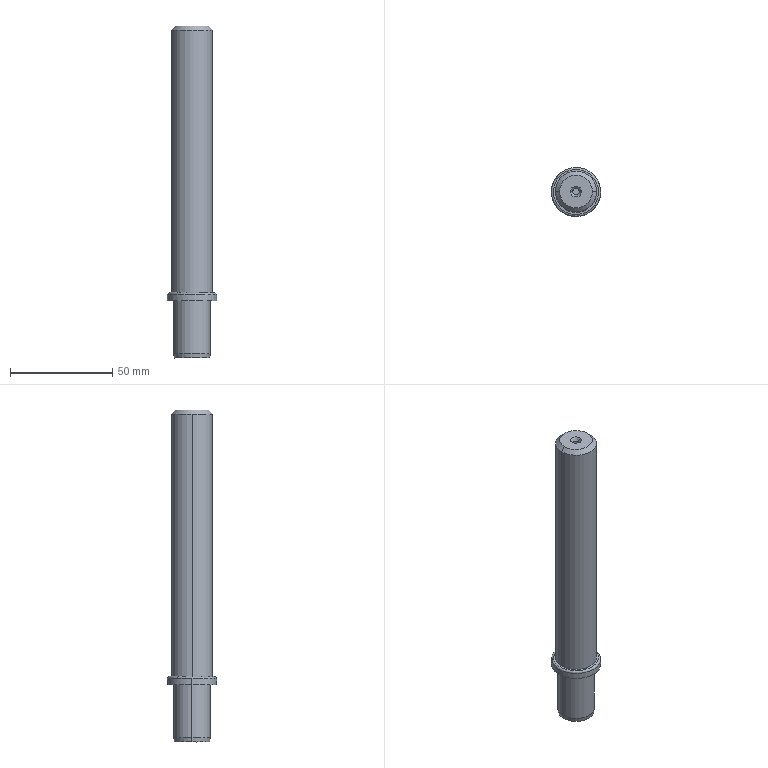Part | SolidWorks | features BaseBody 1 | 1 solid | 33 faces | box 24 x 24 x 162 mm | volume 48875 mm3 | cone 14 | cylinder 12 | plane 5 | spline 2 | commonest cylinder face diameters 3.2 x2 5 x2 6.5 x2 18 x2 20 x2 24 x2
STEP:
#1=CARTESIAN_POINT('',(581.838,-5.206,183.418));
#2=VERTEX_POINT('',#1);
#3=CARTESIAN_POINT('',(599.667,-18.094,183.418));
#4=VERTEX_POINT('',#3);
#5=CARTESIAN_POINT('',(581.838,-5.206,183.418));
#6=CARTESIAN_POINT('',(594.727,12.624,183.418));
#7=CARTESIAN_POINT('',(612.556,-0.265,183.418));
#8=CARTESIAN_POINT('',(599.667,-18.094,183.418));
#9=(BOUNDED_CURVE()B_SPLINE_CURVE(3,(#5,#6,#7,#8),.UNSPECIFIED.,.F.,.F.)B_SPLINE_CURVE_WITH_KNOTS((4,4),(0.,1.),.UNSPECIFIED.)CURVE()GEOMETRIC_REPRESENTATION_ITEM()RATIONAL_B_SPLINE_CURVE((1.,0.3333,0.3333,1.))REPRESENTATION_ITEM(''));
#10=EDGE_CURVE('',#2,#4,#9,.T.);
#11=ORIENTED_EDGE('',*,*,#10,.T.);
#12=CARTESIAN_POINT('',(600.478,-18.68,182.418));
#13=VERTEX_POINT('',#12);
#14=CARTESIAN_POINT('',(599.667,-18.094,182.418));
#15=DIRECTION('',(0.5858,0.8104,0.00000001));
#16=DIRECTION('',(0.8104,-0.5858,0.000000008));
#17=AXIS2_PLACEMENT_3D('',#14,#15,#16);
#18=CIRCLE('',#17,1.);
#19=EDGE_CURVE('',#4,#13,#18,.T.);
#20=ORIENTED_EDGE('',*,*,#19,.T.);
#21=CARTESIAN_POINT('',(602.753,-11.65,182.418));
#22=VERTEX_POINT('',#21);
#23=CARTESIAN_POINT('',(590.753,-11.65,182.418));
#24=DIRECTION('',(-0.000000012,-0.000000003,1.));
#25=DIRECTION('',(-0.8104,0.5858,-0.000000008));
#26=AXIS2_PLACEMENT_3D('',#23,#24,#25);
#27=CIRCLE('',#26,12.);
#28=EDGE_CURVE('',#13,#22,#27,.T.);
#29=ORIENTED_EDGE('',*,*,#28,.T.);
#30=CARTESIAN_POINT('',(581.028,-4.62,182.418));
#31=VERTEX_POINT('',#30);
#32=CARTESIAN_POINT('',(590.753,-11.65,182.418));
#33=DIRECTION('',(-0.000000012,-0.000000003,1.));
#34=DIRECTION('',(-0.8104,0.5858,-0.000000008));
#35=AXIS2_PLACEMENT_3D('',#32,#33,#34);
#36=CIRCLE('',#35,12.);
#37=EDGE_CURVE('',#22,#31,#36,.T.);
#38=ORIENTED_EDGE('',*,*,#37,.T.);
#39=CARTESIAN_POINT('',(581.838,-5.206,182.418));
#40=DIRECTION('',(-0.5858,-0.8104,-0.00000001));
#41=DIRECTION('',(-0.8104,0.5858,-0.000000008));
#42=AXIS2_PLACEMENT_3D('',#39,#40,#41);
#43=CIRCLE('',#42,1.);
#44=EDGE_CURVE('',#2,#31,#43,.T.);
#45=ORIENTED_EDGE('',*,*,#44,.F.);
#46=EDGE_LOOP('',(#11,#20,#29,#38,#45));
#47=FACE_OUTER_BOUND('',#46,.T.);
#48=CARTESIAN_POINT('',(599.667,-18.094,183.418));
#49=CARTESIAN_POINT('',(612.556,-0.265,183.418));
#50=CARTESIAN_POINT('',(594.727,12.624,183.418));
#51=CARTESIAN_POINT('',(581.838,-5.206,183.418));
#52=CARTESIAN_POINT('',(600.142,-18.438,183.418));
#53=CARTESIAN_POINT('',(613.717,0.3413,183.418));
#54=CARTESIAN_POINT('',(594.938,13.916,183.418));
#55=CARTESIAN_POINT('',(581.363,-4.863,183.418));
#56=CARTESIAN_POINT('',(600.478,-18.68,183.004));
#57=CARTESIAN_POINT('',(614.538,0.77,183.004));
#58=CARTESIAN_POINT('',(595.088,14.83,183.004));
#59=CARTESIAN_POINT('',(581.028,-4.62,183.004));
#60=CARTESIAN_POINT('',(600.478,-18.68,182.418));
#61=CARTESIAN_POINT('',(614.538,0.77,182.418));
#62=CARTESIAN_POINT('',(595.088,14.83,182.418));
#63=CARTESIAN_POINT('',(581.028,-4.62,182.418));
#64=(BOUNDED_SURFACE()B_SPLINE_SURFACE(3,3,((#48,#49,#50,#51),(#52,#53,#54,#55),(#56,#57,#58,#59),(#60,#61,#62,#63)),.UNSPECIFIED.,.F.,.F.,.F.)B_SPLINE_SURFACE_WITH_KNOTS((4,4),(4,4),(0.,1.),(0.,1.),.UNSPECIFIED.)GEOMETRIC_REPRESENTATION_ITEM()RATIONAL_B_SPLINE_SURFACE(((1.,0.3333,0.3333,1.),(0.8047,0.2682,0.2682,0.8047),(0.8047,0.2682,0.2682,0.8047),(1.,0.3333,0.3333,1.)))REPRESENTATION_ITEM('')SURFACE());
#65=ADVANCED_FACE('',(#47),#64,.T.);
#66=CARTESIAN_POINT('',(600.753,-11.65,183.418));
#67=VERTEX_POINT('',#66);
#68=CARTESIAN_POINT('',(580.753,-11.65,183.418));
#69=VERTEX_POINT('',#68);
#70=CARTESIAN_POINT('',(590.753,-11.65,183.418));
#71=DIRECTION('',(-0.000000012,-0.000000003,1.));
#72=DIRECTION('',(1.,0.,0.000000012));
#73=AXIS2_PLACEMENT_3D('',#70,#71,#72);
#74=CIRCLE('',#73,10.);
#75=EDGE_CURVE('',#67,#69,#74,.T.);
#76=ORIENTED_EDGE('',*,*,#75,.T.);
#77=CARTESIAN_POINT('',(580.753,-11.65,311.418));
#78=VERTEX_POINT('',#77);
#79=CARTESIAN_POINT('',(580.753,-11.65,321.518));
#80=DIRECTION('',(-0.000000012,-0.000000003,1.));
#81=VECTOR('',#80,1000.);
#82=LINE('',#79,#81);
#83=EDGE_CURVE('',#69,#78,#82,.T.);
#84=ORIENTED_EDGE('',*,*,#83,.T.);
#85=CARTESIAN_POINT('',(600.753,-11.65,311.418));
#86=VERTEX_POINT('',#85);
#87=CARTESIAN_POINT('',(590.753,-11.65,311.418));
#88=DIRECTION('',(0.000000012,0.000000003,-1.));
#89=DIRECTION('',(1.,0.,0.000000012));
#90=AXIS2_PLACEMENT_3D('',#87,#88,#89);
#91=CIRCLE('',#90,10.);
#92=EDGE_CURVE('',#78,#86,#91,.T.);
#93=ORIENTED_EDGE('',*,*,#92,.T.);
#94=CARTESIAN_POINT('',(600.753,-11.65,321.518));
#95=DIRECTION('',(-0.000000012,-0.000000003,1.));
#96=VECTOR('',#95,1000.);
#97=LINE('',#94,#96);
#98=EDGE_CURVE('',#67,#86,#97,.T.);
#99=ORIENTED_EDGE('',*,*,#98,.F.);
#100=EDGE_LOOP('',(#76,#84,#93,#99));
#101=FACE_OUTER_BOUND('',#100,.T.);
#102=CARTESIAN_POINT('',(590.753,-11.65,321.518));
#103=DIRECTION('',(-0.000000012,-0.000000003,1.));
#104=DIRECTION('',(1.,0.,0.000000012));
#105=AXIS2_PLACEMENT_3D('',#102,#103,#104);
#106=CYLINDRICAL_SURFACE('',#105,10.);
#107=ADVANCED_FACE('',(#101),#106,.T.);
#108=CARTESIAN_POINT('',(582.753,-11.65,313.418));
#109=VERTEX_POINT('',#108);
#110=CARTESIAN_POINT('',(598.753,-11.65,313.418));
#111=VERTEX_POINT('',#110);
#112=CARTESIAN_POINT('',(590.753,-11.65,313.418));
#113=DIRECTION('',(0.000000012,0.000000003,-1.));
#114=DIRECTION('',(-1.,0.,-0.000000012));
#115=AXIS2_PLACEMENT_3D('',#112,#113,#114);
#116=CIRCLE('',#115,8.);
#117=EDGE_CURVE('',#109,#111,#116,.T.);
#118=ORIENTED_EDGE('',*,*,#117,.T.);
#119=CARTESIAN_POINT('',(600.753,-11.65,311.418));
#120=DIRECTION('',(0.7071,0.000000002,-0.7071));
#121=VECTOR('',#120,1000.);
#122=LINE('',#119,#121);
#123=EDGE_CURVE('',#111,#86,#122,.T.);
#124=ORIENTED_EDGE('',*,*,#123,.T.);
#125=ORIENTED_EDGE('',*,*,#92,.F.);
#126=CARTESIAN_POINT('',(580.753,-11.65,311.418));
#127=DIRECTION('',(-0.7071,0.000000002,-0.7071));
#128=VECTOR('',#127,1000.);
#129=LINE('',#126,#128);
#130=EDGE_CURVE('',#109,#78,#129,.T.);
#131=ORIENTED_EDGE('',*,*,#130,.F.);
#132=EDGE_LOOP('',(#118,#124,#125,#131));
#133=FACE_OUTER_BOUND('',#132,.T.);
#134=CARTESIAN_POINT('',(590.753,-11.65,311.418));
#135=DIRECTION('',(0.000000012,0.000000003,-1.));
#136=DIRECTION('',(-1.,0.,-0.000000012));
#137=AXIS2_PLACEMENT_3D('',#134,#135,#136);
#138=CONICAL_SURFACE('',#137,10.,0.7854);
#139=ADVANCED_FACE('',(#133),#138,.T.);
#140=CARTESIAN_POINT('',(602.753,-11.65,179.418));
#141=VERTEX_POINT('',#140);
#142=CARTESIAN_POINT('',(578.753,-11.65,179.418));
#143=VERTEX_POINT('',#142);
#144=CARTESIAN_POINT('',(590.753,-11.65,179.418));
#145=DIRECTION('',(-0.000000012,-0.000000003,1.));
#146=DIRECTION('',(1.,0.,0.000000012));
#147=AXIS2_PLACEMENT_3D('',#144,#145,#146);
#148=CIRCLE('',#147,12.);
#149=EDGE_CURVE('',#141,#143,#148,.T.);
#150=ORIENTED_EDGE('',*,*,#149,.T.);
#151=CARTESIAN_POINT('',(578.753,-11.65,182.418));
#152=VERTEX_POINT('',#151);
#153=CARTESIAN_POINT('',(578.753,-11.65,321.518));
#154=DIRECTION('',(-0.000000012,-0.000000003,1.));
#155=VECTOR('',#154,1000.);
#156=LINE('',#153,#155);
#157=EDGE_CURVE('',#143,#152,#156,.T.);
#158=ORIENTED_EDGE('',*,*,#157,.T.);
#159=CARTESIAN_POINT('',(590.753,-11.65,182.418));
#160=DIRECTION('',(-0.000000012,-0.000000003,1.));
#161=DIRECTION('',(-0.8104,0.5858,-0.000000008));
#162=AXIS2_PLACEMENT_3D('',#159,#160,#161);
#163=CIRCLE('',#162,12.);
#164=EDGE_CURVE('',#31,#152,#163,.T.);
#165=ORIENTED_EDGE('',*,*,#164,.F.);
#166=ORIENTED_EDGE('',*,*,#37,.F.);
#167=CARTESIAN_POINT('',(602.753,-11.65,321.518));
#168=DIRECTION('',(-0.000000012,-0.000000003,1.));
#169=VECTOR('',#168,1000.);
#170=LINE('',#167,#169);
#171=EDGE_CURVE('',#141,#22,#170,.T.);
#172=ORIENTED_EDGE('',*,*,#171,.F.);
#173=EDGE_LOOP('',(#150,#158,#165,#166,#172));
#174=FACE_OUTER_BOUND('',#173,.T.);
#175=CARTESIAN_POINT('',(590.753,-11.65,321.518));
#176=DIRECTION('',(-0.000000012,-0.000000003,1.));
#177=DIRECTION('',(1.,0.,0.000000012));
#178=AXIS2_PLACEMENT_3D('',#175,#176,#177);
#179=CYLINDRICAL_SURFACE('',#178,12.);
#180=ADVANCED_FACE('',(#174),#179,.T.);
#181=CARTESIAN_POINT('',(589.153,-11.65,311.599));
#182=VERTEX_POINT('',#181);
#183=CARTESIAN_POINT('',(592.353,-11.65,311.599));
#184=VERTEX_POINT('',#183);
#185=CARTESIAN_POINT('',(590.753,-11.65,311.599));
#186=DIRECTION('',(-0.000000012,-0.000000003,1.));
#187=DIRECTION('',(-0.8104,0.5858,-0.000000008));
#188=AXIS2_PLACEMENT_3D('',#185,#186,#187);
#189=CIRCLE('',#188,1.6);
#190=EDGE_CURVE('',#182,#184,#189,.T.);
#191=ORIENTED_EDGE('',*,*,#190,.F.);
#192=CARTESIAN_POINT('',(588.103,-11.65,313.418));
#193=VERTEX_POINT('',#192);
#194=CARTESIAN_POINT('',(588.103,-11.65,313.418));
#195=DIRECTION('',(-0.5,-0.000000003,0.866));
#196=VECTOR('',#195,1000.);
#197=LINE('',#194,#196);
#198=EDGE_CURVE('',#182,#193,#197,.T.);
#199=ORIENTED_EDGE('',*,*,#198,.T.);
#200=CARTESIAN_POINT('',(593.403,-11.65,313.418));
#201=VERTEX_POINT('',#200);
#202=CARTESIAN_POINT('',(590.753,-11.65,313.418));
#203=DIRECTION('',(-0.000000012,-0.000000003,1.));
#204=DIRECTION('',(1.,0.,0.000000012));
#205=AXIS2_PLACEMENT_3D('',#202,#203,#204);
#206=CIRCLE('',#205,2.65);
#207=EDGE_CURVE('',#193,#201,#206,.T.);
#208=ORIENTED_EDGE('',*,*,#207,.T.);
#209=CARTESIAN_POINT('',(593.403,-11.65,313.418));
#210=DIRECTION('',(0.5,-0.000000003,0.866));
#211=VECTOR('',#210,1000.);
#212=LINE('',#209,#211);
#213=EDGE_CURVE('',#184,#201,#212,.T.);
#214=ORIENTED_EDGE('',*,*,#213,.F.);
#215=EDGE_LOOP('',(#191,#199,#208,#214));
#216=FACE_OUTER_BOUND('',#215,.T.);
#217=CARTESIAN_POINT('',(590.753,-11.65,313.418));
#218=DIRECTION('',(-0.000000012,-0.000000003,1.));
#219=DIRECTION('',(1.,0.,0.000000012));
#220=AXIS2_PLACEMENT_3D('',#217,#218,#219);
#221=CONICAL_SURFACE('',#220,2.65,0.5236);
#222=ADVANCED_FACE('',(#216),#221,.F.);
#223=ORIENTED_EDGE('',*,*,#190,.T.);
#224=CARTESIAN_POINT('',(592.353,-11.65,293.418));
#225=VERTEX_POINT('',#224);
#226=CARTESIAN_POINT('',(592.353,-11.65,313.418));
#227=DIRECTION('',(0.000000012,0.000000003,-1.));
#228=VECTOR('',#227,1000.);
#229=LINE('',#226,#228);
#230=EDGE_CURVE('',#184,#225,#229,.T.);
#231=ORIENTED_EDGE('',*,*,#230,.T.);
#232=CARTESIAN_POINT('',(589.153,-11.65,293.418));
#233=VERTEX_POINT('',#232);
#234=CARTESIAN_POINT('',(590.753,-11.65,293.418));
#235=DIRECTION('',(-0.000000012,-0.000000003,1.));
#236=DIRECTION('',(-1.,0.,-0.000000012));
#237=AXIS2_PLACEMENT_3D('',#234,#235,#236);
#238=CIRCLE('',#237,1.6);
#239=EDGE_CURVE('',#233,#225,#238,.T.);
#240=ORIENTED_EDGE('',*,*,#239,.F.);
#241=CARTESIAN_POINT('',(589.153,-11.65,313.418));
#242=DIRECTION('',(0.000000012,0.000000003,-1.));
#243=VECTOR('',#242,1000.);
#244=LINE('',#241,#243);
#245=EDGE_CURVE('',#182,#233,#244,.T.);
#246=ORIENTED_EDGE('',*,*,#245,.F.);
#247=EDGE_LOOP('',(#223,#231,#240,#246));
#248=FACE_OUTER_BOUND('',#247,.T.);
#249=CARTESIAN_POINT('',(590.753,-11.65,313.418));
#250=DIRECTION('',(0.000000012,0.000000003,-1.));
#251=DIRECTION('',(-1.,0.,-0.000000012));
#252=AXIS2_PLACEMENT_3D('',#249,#250,#251);
#253=CYLINDRICAL_SURFACE('',#252,1.6);
#254=ADVANCED_FACE('',(#248),#253,.F.);
#255=CARTESIAN_POINT('',(599.753,-11.65,153.418));
#256=VERTEX_POINT('',#255);
#257=CARTESIAN_POINT('',(581.753,-11.65,153.418));
#258=VERTEX_POINT('',#257);
#259=CARTESIAN_POINT('',(590.753,-11.65,153.418));
#260=DIRECTION('',(-0.000000012,-0.000000003,1.));
#261=DIRECTION('',(1.,0.,0.000000012));
#262=AXIS2_PLACEMENT_3D('',#259,#260,#261);
#263=CIRCLE('',#262,9.);
#264=EDGE_CURVE('',#256,#258,#263,.T.);
#265=ORIENTED_EDGE('',*,*,#264,.T.);
#266=CARTESIAN_POINT('',(581.753,-11.65,179.418));
#267=VERTEX_POINT('',#266);
#268=CARTESIAN_POINT('',(581.753,-11.65,321.518));
#269=DIRECTION('',(-0.000000012,-0.000000003,1.));
#270=VECTOR('',#269,1000.);
#271=LINE('',#268,#270);
#272=EDGE_CURVE('',#258,#267,#271,.T.);
#273=ORIENTED_EDGE('',*,*,#272,.T.);
#274=CARTESIAN_POINT('',(599.753,-11.65,179.418));
#275=VERTEX_POINT('',#274);
#276=CARTESIAN_POINT('',(590.753,-11.65,179.418));
#277=DIRECTION('',(-0.000000012,-0.000000003,1.));
#278=DIRECTION('',(1.,0.,0.000000012));
#279=AXIS2_PLACEMENT_3D('',#276,#277,#278);
#280=CIRCLE('',#279,9.);
#281=EDGE_CURVE('',#275,#267,#280,.T.);
#282=ORIENTED_EDGE('',*,*,#281,.F.);
#283=CARTESIAN_POINT('',(599.753,-11.65,321.518));
#284=DIRECTION('',(-0.000000012,-0.000000003,1.));
#285=VECTOR('',#284,1000.);
#286=LINE('',#283,#285);
#287=EDGE_CURVE('',#256,#275,#286,.T.);
#288=ORIENTED_EDGE('',*,*,#287,.F.);
#289=EDGE_LOOP('',(#265,#273,#282,#288));
#290=FACE_OUTER_BOUND('',#289,.T.);
#291=CARTESIAN_POINT('',(590.753,-11.65,321.518));
#292=DIRECTION('',(-0.000000012,-0.000000003,1.));
#293=DIRECTION('',(1.,0.,0.000000012));
#294=AXIS2_PLACEMENT_3D('',#291,#292,#293);
#295=CYLINDRICAL_SURFACE('',#294,9.);
#296=ADVANCED_FACE('',(#290),#295,.T.);
#297=CARTESIAN_POINT('',(599.4,-11.65,151.418));
#298=VERTEX_POINT('',#297);
#299=CARTESIAN_POINT('',(582.105,-11.65,151.418));
#300=VERTEX_POINT('',#299);
#301=CARTESIAN_POINT('',(590.753,-11.65,151.418));
#302=DIRECTION('',(-0.000000012,-0.000000003,1.));
#303=DIRECTION('',(1.,0.,0.000000012));
#304=AXIS2_PLACEMENT_3D('',#301,#302,#303);
#305=CIRCLE('',#304,8.647);
#306=EDGE_CURVE('',#298,#300,#305,.T.);
#307=ORIENTED_EDGE('',*,*,#306,.T.);
#308=CARTESIAN_POINT('',(581.753,-11.65,153.418));
#309=DIRECTION('',(-0.1736,-0.000000003,0.9848));
#310=VECTOR('',#309,1000.);
#311=LINE('',#308,#310);
#312=EDGE_CURVE('',#300,#258,#311,.T.);
#313=ORIENTED_EDGE('',*,*,#312,.T.);
#314=ORIENTED_EDGE('',*,*,#264,.F.);
#315=CARTESIAN_POINT('',(599.753,-11.65,153.418));
#316=DIRECTION('',(0.1736,-0.000000003,0.9848));
#317=VECTOR('',#316,1000.);
#318=LINE('',#315,#317);
#319=EDGE_CURVE('',#298,#256,#318,.T.);
#320=ORIENTED_EDGE('',*,*,#319,.F.);
#321=EDGE_LOOP('',(#307,#313,#314,#320));
#322=FACE_OUTER_BOUND('',#321,.T.);
#323=CARTESIAN_POINT('',(590.753,-11.65,153.418));
#324=DIRECTION('',(-0.000000012,-0.000000003,1.));
#325=DIRECTION('',(1.,0.,0.000000012));
#326=AXIS2_PLACEMENT_3D('',#323,#324,#325);
#327=CONICAL_SURFACE('',#326,9.,0.1745);
#328=ADVANCED_FACE('',(#322),#327,.T.);
#329=CARTESIAN_POINT('',(595.003,-11.65,152.573));
#330=VERTEX_POINT('',#329);
#331=CARTESIAN_POINT('',(586.503,-11.65,152.573));
#332=VERTEX_POINT('',#331);
#333=CARTESIAN_POINT('',(590.753,-11.65,152.573));
#334=DIRECTION('',(0.000000012,0.000000003,-1.));
#335=DIRECTION('',(0.8104,-0.5858,0.000000008));
#336=AXIS2_PLACEMENT_3D('',#333,#334,#335);
#337=CIRCLE('',#336,4.25);
#338=EDGE_CURVE('',#330,#332,#337,.T.);
#339=ORIENTED_EDGE('',*,*,#338,.F.);
#340=CARTESIAN_POINT('',(597.003,-11.65,151.418));
#341=VERTEX_POINT('',#340);
#342=CARTESIAN_POINT('',(597.003,-11.65,151.418));
#343=DIRECTION('',(0.866,0.000000002,-0.5));
#344=VECTOR('',#343,1000.);
#345=LINE('',#342,#344);
#346=EDGE_CURVE('',#330,#341,#345,.T.);
#347=ORIENTED_EDGE('',*,*,#346,.T.);
#348=CARTESIAN_POINT('',(584.503,-11.65,151.418));
#349=VERTEX_POINT('',#348);
#350=CARTESIAN_POINT('',(590.753,-11.65,151.418));
#351=DIRECTION('',(-0.000000012,-0.000000003,1.));
#352=DIRECTION('',(-1.,0.,-0.000000012));
#353=AXIS2_PLACEMENT_3D('',#350,#351,#352);
#354=CIRCLE('',#353,6.25);
#355=EDGE_CURVE('',#349,#341,#354,.T.);
#356=ORIENTED_EDGE('',*,*,#355,.F.);
#357=CARTESIAN_POINT('',(584.503,-11.65,151.418));
#358=DIRECTION('',(-0.866,0.000000002,-0.5));
#359=VECTOR('',#358,1000.);
#360=LINE('',#357,#359);
#361=EDGE_CURVE('',#332,#349,#360,.T.);
#362=ORIENTED_EDGE('',*,*,#361,.F.);
#363=EDGE_LOOP('',(#339,#347,#356,#362));
#364=FACE_OUTER_BOUND('',#363,.T.);
#365=CARTESIAN_POINT('',(590.753,-11.65,151.418));
#366=DIRECTION('',(0.000000012,0.000000003,-1.));
#367=DIRECTION('',(-1.,0.,-0.000000012));
#368=AXIS2_PLACEMENT_3D('',#365,#366,#367);
#369=CONICAL_SURFACE('',#368,6.25,1.047);
#370=ADVANCED_FACE('',(#364),#369,.F.);
#371=CARTESIAN_POINT('',(594.003,-11.65,154.305));
#372=VERTEX_POINT('',#371);
#373=CARTESIAN_POINT('',(587.503,-11.65,154.305));
#374=VERTEX_POINT('',#373);
#375=CARTESIAN_POINT('',(590.753,-11.65,154.305));
#376=DIRECTION('',(0.000000012,0.000000003,-1.));
#377=DIRECTION('',(0.8104,-0.5858,0.000000008));
#378=AXIS2_PLACEMENT_3D('',#375,#376,#377);
#379=CIRCLE('',#378,3.25);
#380=EDGE_CURVE('',#372,#374,#379,.T.);
#381=ORIENTED_EDGE('',*,*,#380,.F.);
#382=CARTESIAN_POINT('',(595.003,-11.65,152.573));
#383=DIRECTION('',(0.5,0.000000003,-0.866));
#384=VECTOR('',#383,1000.);
#385=LINE('',#382,#384);
#386=EDGE_CURVE('',#372,#330,#385,.T.);
#387=ORIENTED_EDGE('',*,*,#386,.T.);
#388=ORIENTED_EDGE('',*,*,#338,.T.);
#389=CARTESIAN_POINT('',(586.503,-11.65,152.573));
#390=DIRECTION('',(-0.5,0.000000003,-0.866));
#391=VECTOR('',#390,1000.);
#392=LINE('',#389,#391);
#393=EDGE_CURVE('',#374,#332,#392,.T.);
#394=ORIENTED_EDGE('',*,*,#393,.F.);
#395=EDGE_LOOP('',(#381,#387,#388,#394));
#396=FACE_OUTER_BOUND('',#395,.T.);
#397=CARTESIAN_POINT('',(590.753,-11.65,152.573));
#398=DIRECTION('',(0.000000012,0.000000003,-1.));
#399=DIRECTION('',(-1.,0.,-0.000000012));
#400=AXIS2_PLACEMENT_3D('',#397,#398,#399);
#401=CONICAL_SURFACE('',#400,4.25,0.5236);
#402=ADVANCED_FACE('',(#396),#401,.F.);
#403=ORIENTED_EDGE('',*,*,#380,.T.);
#404=CARTESIAN_POINT('',(587.503,-11.65,156.418));
#405=VERTEX_POINT('',#404);
#406=CARTESIAN_POINT('',(587.503,-11.65,174.984));
#407=DIRECTION('',(-0.000000012,-0.000000003,1.));
#408=VECTOR('',#407,1000.);
#409=LINE('',#406,#408);
#410=EDGE_CURVE('',#374,#405,#409,.T.);
#411=ORIENTED_EDGE('',*,*,#410,.T.);
#412=CARTESIAN_POINT('',(594.003,-11.65,156.418));
#413=VERTEX_POINT('',#412);
#414=CARTESIAN_POINT('',(590.753,-11.65,156.418));
#415=DIRECTION('',(0.000000012,0.000000003,-1.));
#416=DIRECTION('',(1.,0.,0.000000012));
#417=AXIS2_PLACEMENT_3D('',#414,#415,#416);
#418=CIRCLE('',#417,3.25);
#419=EDGE_CURVE('',#413,#405,#418,.T.);
#420=ORIENTED_EDGE('',*,*,#419,.F.);
#421=CARTESIAN_POINT('',(594.003,-11.65,174.984));
#422=DIRECTION('',(-0.000000012,-0.000000003,1.));
#423=VECTOR('',#422,1000.);
#424=LINE('',#421,#423);
#425=EDGE_CURVE('',#372,#413,#424,.T.);
#426=ORIENTED_EDGE('',*,*,#425,.F.);
#427=EDGE_LOOP('',(#403,#411,#420,#426));
#428=FACE_OUTER_BOUND('',#427,.T.);
#429=CARTESIAN_POINT('',(590.753,-11.65,174.984));
#430=DIRECTION('',(-0.000000012,-0.000000003,1.));
#431=DIRECTION('',(1.,0.,0.000000012));
#432=AXIS2_PLACEMENT_3D('',#429,#430,#431);
#433=CYLINDRICAL_SURFACE('',#432,3.25);
#434=ADVANCED_FACE('',(#428),#433,.F.);
#435=CARTESIAN_POINT('',(593.253,-11.65,156.851));
#436=VERTEX_POINT('',#435);
#437=CARTESIAN_POINT('',(588.253,-11.65,156.851));
#438=VERTEX_POINT('',#437);
#439=CARTESIAN_POINT('',(590.753,-11.65,156.851));
#440=DIRECTION('',(0.000000012,0.000000003,-1.));
#441=DIRECTION('',(0.8104,-0.5858,0.000000008));
#442=AXIS2_PLACEMENT_3D('',#439,#440,#441);
#443=CIRCLE('',#442,2.5);
#444=EDGE_CURVE('',#436,#438,#443,.T.);
#445=ORIENTED_EDGE('',*,*,#444,.F.);
#446=CARTESIAN_POINT('',(594.003,-11.65,156.418));
#447=DIRECTION('',(0.866,0.000000002,-0.5));
#448=VECTOR('',#447,1000.);
#449=LINE('',#446,#448);
#450=EDGE_CURVE('',#436,#413,#449,.T.);
#451=ORIENTED_EDGE('',*,*,#450,.T.);
#452=ORIENTED_EDGE('',*,*,#419,.T.);
#453=CARTESIAN_POINT('',(587.503,-11.65,156.418));
#454=DIRECTION('',(-0.866,0.000000002,-0.5));
#455=VECTOR('',#454,1000.);
#456=LINE('',#453,#455);
#457=EDGE_CURVE('',#438,#405,#456,.T.);
#458=ORIENTED_EDGE('',*,*,#457,.F.);
#459=EDGE_LOOP('',(#445,#451,#452,#458));
#460=FACE_OUTER_BOUND('',#459,.T.);
#461=CARTESIAN_POINT('',(590.753,-11.65,156.418));
#462=DIRECTION('',(0.000000012,0.000000003,-1.));
#463=DIRECTION('',(-1.,0.,-0.000000012));
#464=AXIS2_PLACEMENT_3D('',#461,#462,#463);
#465=CONICAL_SURFACE('',#464,3.25,1.047);
#466=ADVANCED_FACE('',(#460),#465,.F.);
#467=ORIENTED_EDGE('',*,*,#444,.T.);
#468=CARTESIAN_POINT('',(588.253,-11.65,172.418));
#469=VERTEX_POINT('',#468);
#470=CARTESIAN_POINT('',(588.253,-11.65,174.984));
#471=DIRECTION('',(-0.000000012,-0.000000003,1.));
#472=VECTOR('',#471,1000.);
#473=LINE('',#470,#472);
#474=EDGE_CURVE('',#438,#469,#473,.T.);
#475=ORIENTED_EDGE('',*,*,#474,.T.);
#476=CARTESIAN_POINT('',(593.253,-11.65,172.418));
#477=VERTEX_POINT('',#476);
#478=CARTESIAN_POINT('',(590.753,-11.65,172.418));
#479=DIRECTION('',(0.000000012,0.000000003,-1.));
#480=DIRECTION('',(1.,0.,0.000000012));
#481=AXIS2_PLACEMENT_3D('',#478,#479,#480);
#482=CIRCLE('',#481,2.5);
#483=EDGE_CURVE('',#477,#469,#482,.T.);
#484=ORIENTED_EDGE('',*,*,#483,.F.);
#485=CARTESIAN_POINT('',(593.253,-11.65,174.984));
#486=DIRECTION('',(-0.000000012,-0.000000003,1.));
#487=VECTOR('',#486,1000.);
#488=LINE('',#485,#487);
#489=EDGE_CURVE('',#436,#477,#488,.T.);
#490=ORIENTED_EDGE('',*,*,#489,.F.);
#491=EDGE_LOOP('',(#467,#475,#484,#490));
#492=FACE_OUTER_BOUND('',#491,.T.);
#493=CARTESIAN_POINT('',(590.753,-11.65,174.984));
#494=DIRECTION('',(-0.000000012,-0.000000003,1.));
#495=DIRECTION('',(1.,0.,0.000000012));
#496=AXIS2_PLACEMENT_3D('',#493,#494,#495);
#497=CYLINDRICAL_SURFACE('',#496,2.5);
#498=ADVANCED_FACE('',(#492),#497,.F.);
#499=CARTESIAN_POINT('',(590.753,-11.65,173.862));
#500=VERTEX_POINT('',#499);
#501=CARTESIAN_POINT('',(588.253,-11.65,172.418));
#502=DIRECTION('',(-0.866,0.000000002,-0.5));
#503=VECTOR('',#502,1000.);
#504=LINE('',#501,#503);
#505=EDGE_CURVE('',#500,#469,#504,.T.);
#506=ORIENTED_EDGE('',*,*,#505,.F.);
#507=CARTESIAN_POINT('',(593.253,-11.65,172.418));
#508=DIRECTION('',(0.866,0.000000002,-0.5));
#509=VECTOR('',#508,1000.);
#510=LINE('',#507,#509);
#511=EDGE_CURVE('',#500,#477,#510,.T.);
#512=ORIENTED_EDGE('',*,*,#511,.T.);
#513=ORIENTED_EDGE('',*,*,#483,.T.);
#514=EDGE_LOOP('',(#506,#512,#513));
#515=FACE_OUTER_BOUND('',#514,.T.);
#516=CARTESIAN_POINT('',(590.753,-11.65,172.418));
#517=DIRECTION('',(0.000000012,0.000000003,-1.));
#518=DIRECTION('',(-1.,0.,-0.000000012));
#519=AXIS2_PLACEMENT_3D('',#516,#517,#518);
#520=CONICAL_SURFACE('',#519,2.5,1.047);
#521=ADVANCED_FACE('',(#515),#520,.F.);
#522=ORIENTED_EDGE('',*,*,#83,.F.);
#523=CARTESIAN_POINT('',(590.753,-11.65,183.418));
#524=DIRECTION('',(-0.000000012,-0.000000003,1.));
#525=DIRECTION('',(1.,0.,0.000000012));
#526=AXIS2_PLACEMENT_3D('',#523,#524,#525);
#527=CIRCLE('',#526,10.);
#528=EDGE_CURVE('',#69,#67,#527,.T.);
#529=ORIENTED_EDGE('',*,*,#528,.T.);
#530=ORIENTED_EDGE('',*,*,#98,.T.);
#531=CARTESIAN_POINT('',(590.753,-11.65,311.418));
#532=DIRECTION('',(0.000000012,0.000000003,-1.));
#533=DIRECTION('',(1.,0.,0.000000012));
#534=AXIS2_PLACEMENT_3D('',#531,#532,#533);
#535=CIRCLE('',#534,10.);
#536=EDGE_CURVE('',#86,#78,#535,.T.);
#537=ORIENTED_EDGE('',*,*,#536,.T.);
#538=EDGE_LOOP('',(#522,#529,#530,#537));
#539=FACE_OUTER_BOUND('',#538,.T.);
#540=CARTESIAN_POINT('',(590.753,-11.65,321.518));
#541=DIRECTION('',(-0.000000012,-0.000000003,1.));
#542=DIRECTION('',(1.,0.,0.000000012));
#543=AXIS2_PLACEMENT_3D('',#540,#541,#542);
#544=CYLINDRICAL_SURFACE('',#543,10.);
#545=ADVANCED_FACE('',(#539),#544,.T.);
#546=ORIENTED_EDGE('',*,*,#10,.F.);
#547=CARTESIAN_POINT('',(599.667,-18.094,183.418));
#548=CARTESIAN_POINT('',(586.779,-35.924,183.418));
#549=CARTESIAN_POINT('',(568.95,-23.035,183.418));
#550=CARTESIAN_POINT('',(581.838,-5.206,183.418));
#551=(BOUNDED_CURVE()B_SPLINE_CURVE(3,(#547,#548,#549,#550),.UNSPECIFIED.,.F.,.F.)B_SPLINE_CURVE_WITH_KNOTS((4,4),(0.,1.),.UNSPECIFIED.)CURVE()GEOMETRIC_REPRESENTATION_ITEM()RATIONAL_B_SPLINE_CURVE((1.,0.3333,0.3333,1.))REPRESENTATION_ITEM(''));
#552=EDGE_CURVE('',#4,#2,#551,.T.);
#553=ORIENTED_EDGE('',*,*,#552,.F.);
#554=EDGE_LOOP('',(#546,#553));
#555=FACE_OUTER_BOUND('',#554,.T.);
#556=ORIENTED_EDGE('',*,*,#75,.F.);
#557=ORIENTED_EDGE('',*,*,#528,.F.);
#558=EDGE_LOOP('',(#556,#557));
#559=FACE_BOUND('',#558,.T.);
#560=CARTESIAN_POINT('',(590.753,-11.65,183.418));
#561=DIRECTION('',(0.000000012,0.000000003,-1.));
#562=DIRECTION('',(-1.,0.,-0.000000012));
#563=AXIS2_PLACEMENT_3D('',#560,#561,#562);
#564=PLANE('',#563);
#565=ADVANCED_FACE('',(#555,#559),#564,.F.);
#566=ORIENTED_EDGE('',*,*,#123,.F.);
#567=CARTESIAN_POINT('',(590.753,-11.65,313.418));
#568=DIRECTION('',(0.000000012,0.000000003,-1.));
#569=DIRECTION('',(-1.,0.,-0.000000012));
#570=AXIS2_PLACEMENT_3D('',#567,#568,#569);
#571=CIRCLE('',#570,8.);
#572=EDGE_CURVE('',#111,#109,#571,.T.);
#573=ORIENTED_EDGE('',*,*,#572,.T.);
#574=ORIENTED_EDGE('',*,*,#130,.T.);
#575=ORIENTED_EDGE('',*,*,#536,.F.);
#576=EDGE_LOOP('',(#566,#573,#574,#575));
#577=FACE_OUTER_BOUND('',#576,.T.);
#578=CARTESIAN_POINT('',(590.753,-11.65,311.418));
#579=DIRECTION('',(0.000000012,0.000000003,-1.));
#580=DIRECTION('',(-1.,0.,-0.000000012));
#581=AXIS2_PLACEMENT_3D('',#578,#579,#580);
#582=CONICAL_SURFACE('',#581,10.,0.7854);
#583=ADVANCED_FACE('',(#577),#582,.T.);
#584=ORIENTED_EDGE('',*,*,#19,.F.);
#585=ORIENTED_EDGE('',*,*,#552,.T.);
#586=ORIENTED_EDGE('',*,*,#44,.T.);
#587=ORIENTED_EDGE('',*,*,#164,.T.);
#588=CARTESIAN_POINT('',(590.753,-11.65,182.418));
#589=DIRECTION('',(-0.000000012,-0.000000003,1.));
#590=DIRECTION('',(-0.8104,0.5858,-0.000000008));
#591=AXIS2_PLACEMENT_3D('',#588,#589,#590);
#592=CIRCLE('',#591,12.);
#593=EDGE_CURVE('',#152,#13,#592,.T.);
#594=ORIENTED_EDGE('',*,*,#593,.T.);
#595=EDGE_LOOP('',(#584,#585,#586,#587,#594));
#596=FACE_OUTER_BOUND('',#595,.T.);
#597=CARTESIAN_POINT('',(581.838,-5.206,183.418));
#598=CARTESIAN_POINT('',(568.95,-23.035,183.418));
#599=CARTESIAN_POINT('',(586.779,-35.924,183.418));
#600=CARTESIAN_POINT('',(599.667,-18.094,183.418));
#601=CARTESIAN_POINT('',(581.363,-4.863,183.418));
#602=CARTESIAN_POINT('',(567.788,-23.641,183.418));
#603=CARTESIAN_POINT('',(586.567,-37.216,183.418));
#604=CARTESIAN_POINT('',(600.142,-18.438,183.418));
#605=CARTESIAN_POINT('',(581.028,-4.62,183.004));
#606=CARTESIAN_POINT('',(566.967,-24.07,183.004));
#607=CARTESIAN_POINT('',(586.418,-38.13,183.004));
#608=CARTESIAN_POINT('',(600.478,-18.68,183.004));
#609=CARTESIAN_POINT('',(581.028,-4.62,182.418));
#610=CARTESIAN_POINT('',(566.967,-24.07,182.418));
#611=CARTESIAN_POINT('',(586.418,-38.13,182.418));
#612=CARTESIAN_POINT('',(600.478,-18.68,182.418));
#613=(BOUNDED_SURFACE()B_SPLINE_SURFACE(3,3,((#597,#598,#599,#600),(#601,#602,#603,#604),(#605,#606,#607,#608),(#609,#610,#611,#612)),.UNSPECIFIED.,.F.,.F.,.F.)B_SPLINE_SURFACE_WITH_KNOTS((4,4),(4,4),(0.,1.),(0.,1.),.UNSPECIFIED.)GEOMETRIC_REPRESENTATION_ITEM()RATIONAL_B_SPLINE_SURFACE(((1.,0.3333,0.3333,1.),(0.8047,0.2682,0.2682,0.8047),(0.8047,0.2682,0.2682,0.8047),(1.,0.3333,0.3333,1.)))REPRESENTATION_ITEM('')SURFACE());
#614=ADVANCED_FACE('',(#596),#613,.T.);
#615=CARTESIAN_POINT('',(590.753,-11.65,313.418));
#616=DIRECTION('',(-0.000000012,-0.000000003,1.));
#617=DIRECTION('',(1.,0.,0.000000012));
#618=AXIS2_PLACEMENT_3D('',#615,#616,#617);
#619=CIRCLE('',#618,2.65);
#620=EDGE_CURVE('',#201,#193,#619,.T.);
#621=ORIENTED_EDGE('',*,*,#620,.F.);
#622=ORIENTED_EDGE('',*,*,#207,.F.);
#623=EDGE_LOOP('',(#621,#622));
#624=FACE_BOUND('',#623,.T.);
#625=ORIENTED_EDGE('',*,*,#117,.F.);
#626=ORIENTED_EDGE('',*,*,#572,.F.);
#627=EDGE_LOOP('',(#625,#626));
#628=FACE_OUTER_BOUND('',#627,.T.);
#629=CARTESIAN_POINT('',(590.753,-11.65,313.418));
#630=DIRECTION('',(0.000000012,0.000000003,-1.));
#631=DIRECTION('',(-1.,0.,-0.000000012));
#632=AXIS2_PLACEMENT_3D('',#629,#630,#631);
#633=PLANE('',#632);
#634=ADVANCED_FACE('',(#624,#628),#633,.F.);
#635=ORIENTED_EDGE('',*,*,#157,.F.);
#636=CARTESIAN_POINT('',(590.753,-11.65,179.418));
#637=DIRECTION('',(-0.000000012,-0.000000003,1.));
#638=DIRECTION('',(1.,0.,0.000000012));
#639=AXIS2_PLACEMENT_3D('',#636,#637,#638);
#640=CIRCLE('',#639,12.);
#641=EDGE_CURVE('',#143,#141,#640,.T.);
#642=ORIENTED_EDGE('',*,*,#641,.T.);
#643=ORIENTED_EDGE('',*,*,#171,.T.);
#644=ORIENTED_EDGE('',*,*,#28,.F.);
#645=ORIENTED_EDGE('',*,*,#593,.F.);
#646=EDGE_LOOP('',(#635,#642,#643,#644,#645));
#647=FACE_OUTER_BOUND('',#646,.T.);
#648=CARTESIAN_POINT('',(590.753,-11.65,321.518));
#649=DIRECTION('',(-0.000000012,-0.000000003,1.));
#650=DIRECTION('',(1.,0.,0.000000012));
#651=AXIS2_PLACEMENT_3D('',#648,#649,#650);
#652=CYLINDRICAL_SURFACE('',#651,12.);
#653=ADVANCED_FACE('',(#647),#652,.T.);
#654=ORIENTED_EDGE('',*,*,#198,.F.);
#655=CARTESIAN_POINT('',(590.753,-11.65,311.599));
#656=DIRECTION('',(-0.000000012,-0.000000003,1.));
#657=DIRECTION('',(-0.8104,0.5858,-0.000000008));
#658=AXIS2_PLACEMENT_3D('',#655,#656,#657);
#659=CIRCLE('',#658,1.6);
#660=EDGE_CURVE('',#184,#182,#659,.T.);
#661=ORIENTED_EDGE('',*,*,#660,.F.);
#662=ORIENTED_EDGE('',*,*,#213,.T.);
#663=ORIENTED_EDGE('',*,*,#620,.T.);
#664=EDGE_LOOP('',(#654,#661,#662,#663));
#665=FACE_OUTER_BOUND('',#664,.T.);
#666=CARTESIAN_POINT('',(590.753,-11.65,313.418));
#667=DIRECTION('',(-0.000000012,-0.000000003,1.));
#668=DIRECTION('',(1.,0.,0.000000012));
#669=AXIS2_PLACEMENT_3D('',#666,#667,#668);
#670=CONICAL_SURFACE('',#669,2.65,0.5236);
#671=ADVANCED_FACE('',(#665),#670,.F.);
#672=ORIENTED_EDGE('',*,*,#281,.T.);
#673=CARTESIAN_POINT('',(590.753,-11.65,179.418));
#674=DIRECTION('',(-0.000000012,-0.000000003,1.));
#675=DIRECTION('',(1.,0.,0.000000012));
#676=AXIS2_PLACEMENT_3D('',#673,#674,#675);
#677=CIRCLE('',#676,9.);
#678=EDGE_CURVE('',#267,#275,#677,.T.);
#679=ORIENTED_EDGE('',*,*,#678,.T.);
#680=EDGE_LOOP('',(#672,#679));
#681=FACE_BOUND('',#680,.T.);
#682=ORIENTED_EDGE('',*,*,#149,.F.);
#683=ORIENTED_EDGE('',*,*,#641,.F.);
#684=EDGE_LOOP('',(#682,#683));
#685=FACE_OUTER_BOUND('',#684,.T.);
#686=CARTESIAN_POINT('',(590.753,-11.65,179.418));
#687=DIRECTION('',(0.000000012,0.000000003,-1.));
#688=DIRECTION('',(-1.,0.,-0.000000012));
#689=AXIS2_PLACEMENT_3D('',#686,#687,#688);
#690=PLANE('',#689);
#691=ADVANCED_FACE('',(#681,#685),#690,.T.);
#692=ORIENTED_EDGE('',*,*,#230,.F.);
#693=ORIENTED_EDGE('',*,*,#660,.T.);
#694=ORIENTED_EDGE('',*,*,#245,.T.);
#695=CARTESIAN_POINT('',(590.753,-11.65,293.418));
#696=DIRECTION('',(-0.000000012,-0.000000003,1.));
#697=DIRECTION('',(-1.,0.,-0.000000012));
#698=AXIS2_PLACEMENT_3D('',#695,#696,#697);
#699=CIRCLE('',#698,1.6);
#700=EDGE_CURVE('',#225,#233,#699,.T.);
#701=ORIENTED_EDGE('',*,*,#700,.F.);
#702=EDGE_LOOP('',(#692,#693,#694,#701));
#703=FACE_OUTER_BOUND('',#702,.T.);
#704=CARTESIAN_POINT('',(590.753,-11.65,313.418));
#705=DIRECTION('',(0.000000012,0.000000003,-1.));
#706=DIRECTION('',(-1.,0.,-0.000000012));
#707=AXIS2_PLACEMENT_3D('',#704,#705,#706);
#708=CYLINDRICAL_SURFACE('',#707,1.6);
#709=ADVANCED_FACE('',(#703),#708,.F.);
#710=ORIENTED_EDGE('',*,*,#272,.F.);
#711=CARTESIAN_POINT('',(590.753,-11.65,153.418));
#712=DIRECTION('',(-0.000000012,-0.000000003,1.));
#713=DIRECTION('',(1.,0.,0.000000012));
#714=AXIS2_PLACEMENT_3D('',#711,#712,#713);
#715=CIRCLE('',#714,9.);
#716=EDGE_CURVE('',#258,#256,#715,.T.);
#717=ORIENTED_EDGE('',*,*,#716,.T.);
#718=ORIENTED_EDGE('',*,*,#287,.T.);
#719=ORIENTED_EDGE('',*,*,#678,.F.);
#720=EDGE_LOOP('',(#710,#717,#718,#719));
#721=FACE_OUTER_BOUND('',#720,.T.);
#722=CARTESIAN_POINT('',(590.753,-11.65,321.518));
#723=DIRECTION('',(-0.000000012,-0.000000003,1.));
#724=DIRECTION('',(1.,0.,0.000000012));
#725=AXIS2_PLACEMENT_3D('',#722,#723,#724);
#726=CYLINDRICAL_SURFACE('',#725,9.);
#727=ADVANCED_FACE('',(#721),#726,.T.);
#728=ORIENTED_EDGE('',*,*,#239,.T.);
#729=ORIENTED_EDGE('',*,*,#700,.T.);
#730=EDGE_LOOP('',(#728,#729));
#731=FACE_OUTER_BOUND('',#730,.T.);
#732=CARTESIAN_POINT('',(590.753,-11.65,293.418));
#733=DIRECTION('',(0.000000012,0.000000003,-1.));
#734=DIRECTION('',(-1.,0.,-0.000000012));
#735=AXIS2_PLACEMENT_3D('',#732,#733,#734);
#736=PLANE('',#735);
#737=ADVANCED_FACE('',(#731),#736,.F.);
#738=ORIENTED_EDGE('',*,*,#312,.F.);
#739=CARTESIAN_POINT('',(590.753,-11.65,151.418));
#740=DIRECTION('',(-0.000000012,-0.000000003,1.));
#741=DIRECTION('',(1.,0.,0.000000012));
#742=AXIS2_PLACEMENT_3D('',#739,#740,#741);
#743=CIRCLE('',#742,8.647);
#744=EDGE_CURVE('',#300,#298,#743,.T.);
#745=ORIENTED_EDGE('',*,*,#744,.T.);
#746=ORIENTED_EDGE('',*,*,#319,.T.);
#747=ORIENTED_EDGE('',*,*,#716,.F.);
#748=EDGE_LOOP('',(#738,#745,#746,#747));
#749=FACE_OUTER_BOUND('',#748,.T.);
#750=CARTESIAN_POINT('',(590.753,-11.65,153.418));
#751=DIRECTION('',(-0.000000012,-0.000000003,1.));
#752=DIRECTION('',(1.,0.,0.000000012));
#753=AXIS2_PLACEMENT_3D('',#750,#751,#752);
#754=CONICAL_SURFACE('',#753,9.,0.1745);
#755=ADVANCED_FACE('',(#749),#754,.T.);
#756=ORIENTED_EDGE('',*,*,#355,.T.);
#757=CARTESIAN_POINT('',(590.753,-11.65,151.418));
#758=DIRECTION('',(-0.000000012,-0.000000003,1.));
#759=DIRECTION('',(-1.,0.,-0.000000012));
#760=AXIS2_PLACEMENT_3D('',#757,#758,#759);
#761=CIRCLE('',#760,6.25);
#762=EDGE_CURVE('',#341,#349,#761,.T.);
#763=ORIENTED_EDGE('',*,*,#762,.T.);
#764=EDGE_LOOP('',(#756,#763));
#765=FACE_BOUND('',#764,.T.);
#766=ORIENTED_EDGE('',*,*,#306,.F.);
#767=ORIENTED_EDGE('',*,*,#744,.F.);
#768=EDGE_LOOP('',(#766,#767));
#769=FACE_OUTER_BOUND('',#768,.T.);
#770=CARTESIAN_POINT('',(590.753,-11.65,151.418));
#771=DIRECTION('',(0.000000012,0.000000003,-1.));
#772=DIRECTION('',(-1.,0.,-0.000000012));
#773=AXIS2_PLACEMENT_3D('',#770,#771,#772);
#774=PLANE('',#773);
#775=ADVANCED_FACE('',(#765,#769),#774,.T.);
#776=ORIENTED_EDGE('',*,*,#346,.F.);
#777=CARTESIAN_POINT('',(590.753,-11.65,152.573));
#778=DIRECTION('',(0.000000012,0.000000003,-1.));
#779=DIRECTION('',(0.8104,-0.5858,0.000000008));
#780=AXIS2_PLACEMENT_3D('',#777,#778,#779);
#781=CIRCLE('',#780,4.25);
#782=EDGE_CURVE('',#332,#330,#781,.T.);
#783=ORIENTED_EDGE('',*,*,#782,.F.);
#784=ORIENTED_EDGE('',*,*,#361,.T.);
#785=ORIENTED_EDGE('',*,*,#762,.F.);
#786=EDGE_LOOP('',(#776,#783,#784,#785));
#787=FACE_OUTER_BOUND('',#786,.T.);
#788=CARTESIAN_POINT('',(590.753,-11.65,151.418));
#789=DIRECTION('',(0.000000012,0.000000003,-1.));
#790=DIRECTION('',(-1.,0.,-0.000000012));
#791=AXIS2_PLACEMENT_3D('',#788,#789,#790);
#792=CONICAL_SURFACE('',#791,6.25,1.047);
#793=ADVANCED_FACE('',(#787),#792,.F.);
#794=ORIENTED_EDGE('',*,*,#386,.F.);
#795=CARTESIAN_POINT('',(590.753,-11.65,154.305));
#796=DIRECTION('',(0.000000012,0.000000003,-1.));
#797=DIRECTION('',(0.8104,-0.5858,0.000000008));
#798=AXIS2_PLACEMENT_3D('',#795,#796,#797);
#799=CIRCLE('',#798,3.25);
#800=EDGE_CURVE('',#374,#372,#799,.T.);
#801=ORIENTED_EDGE('',*,*,#800,.F.);
#802=ORIENTED_EDGE('',*,*,#393,.T.);
#803=ORIENTED_EDGE('',*,*,#782,.T.);
#804=EDGE_LOOP('',(#794,#801,#802,#803));
#805=FACE_OUTER_BOUND('',#804,.T.);
#806=CARTESIAN_POINT('',(590.753,-11.65,152.573));
#807=DIRECTION('',(0.000000012,0.000000003,-1.));
#808=DIRECTION('',(-1.,0.,-0.000000012));
#809=AXIS2_PLACEMENT_3D('',#806,#807,#808);
#810=CONICAL_SURFACE('',#809,4.25,0.5236);
#811=ADVANCED_FACE('',(#805),#810,.F.);
#812=ORIENTED_EDGE('',*,*,#410,.F.);
#813=ORIENTED_EDGE('',*,*,#800,.T.);
#814=ORIENTED_EDGE('',*,*,#425,.T.);
#815=CARTESIAN_POINT('',(590.753,-11.65,156.418));
#816=DIRECTION('',(0.000000012,0.000000003,-1.));
#817=DIRECTION('',(1.,0.,0.000000012));
#818=AXIS2_PLACEMENT_3D('',#815,#816,#817);
#819=CIRCLE('',#818,3.25);
#820=EDGE_CURVE('',#405,#413,#819,.T.);
#821=ORIENTED_EDGE('',*,*,#820,.F.);
#822=EDGE_LOOP('',(#812,#813,#814,#821));
#823=FACE_OUTER_BOUND('',#822,.T.);
#824=CARTESIAN_POINT('',(590.753,-11.65,174.984));
#825=DIRECTION('',(-0.000000012,-0.000000003,1.));
#826=DIRECTION('',(1.,0.,0.000000012));
#827=AXIS2_PLACEMENT_3D('',#824,#825,#826);
#828=CYLINDRICAL_SURFACE('',#827,3.25);
#829=ADVANCED_FACE('',(#823),#828,.F.);
#830=ORIENTED_EDGE('',*,*,#450,.F.);
#831=CARTESIAN_POINT('',(590.753,-11.65,156.851));
#832=DIRECTION('',(0.000000012,0.000000003,-1.));
#833=DIRECTION('',(0.8104,-0.5858,0.000000008));
#834=AXIS2_PLACEMENT_3D('',#831,#832,#833);
#835=CIRCLE('',#834,2.5);
#836=EDGE_CURVE('',#438,#436,#835,.T.);
#837=ORIENTED_EDGE('',*,*,#836,.F.);
#838=ORIENTED_EDGE('',*,*,#457,.T.);
#839=ORIENTED_EDGE('',*,*,#820,.T.);
#840=EDGE_LOOP('',(#830,#837,#838,#839));
#841=FACE_OUTER_BOUND('',#840,.T.);
#842=CARTESIAN_POINT('',(590.753,-11.65,156.418));
#843=DIRECTION('',(0.000000012,0.000000003,-1.));
#844=DIRECTION('',(-1.,0.,-0.000000012));
#845=AXIS2_PLACEMENT_3D('',#842,#843,#844);
#846=CONICAL_SURFACE('',#845,3.25,1.047);
#847=ADVANCED_FACE('',(#841),#846,.F.);
#848=ORIENTED_EDGE('',*,*,#474,.F.);
#849=ORIENTED_EDGE('',*,*,#836,.T.);
#850=ORIENTED_EDGE('',*,*,#489,.T.);
#851=CARTESIAN_POINT('',(590.753,-11.65,172.418));
#852=DIRECTION('',(0.000000012,0.000000003,-1.));
#853=DIRECTION('',(1.,0.,0.000000012));
#854=AXIS2_PLACEMENT_3D('',#851,#852,#853);
#855=CIRCLE('',#854,2.5);
#856=EDGE_CURVE('',#469,#477,#855,.T.);
#857=ORIENTED_EDGE('',*,*,#856,.F.);
#858=EDGE_LOOP('',(#848,#849,#850,#857));
#859=FACE_OUTER_BOUND('',#858,.T.);
#860=CARTESIAN_POINT('',(590.753,-11.65,174.984));
#861=DIRECTION('',(-0.000000012,-0.000000003,1.));
#862=DIRECTION('',(1.,0.,0.000000012));
#863=AXIS2_PLACEMENT_3D('',#860,#861,#862);
#864=CYLINDRICAL_SURFACE('',#863,2.5);
#865=ADVANCED_FACE('',(#859),#864,.F.);
#866=ORIENTED_EDGE('',*,*,#511,.F.);
#867=ORIENTED_EDGE('',*,*,#505,.T.);
#868=ORIENTED_EDGE('',*,*,#856,.T.);
#869=EDGE_LOOP('',(#866,#867,#868));
#870=FACE_OUTER_BOUND('',#869,.T.);
#871=CARTESIAN_POINT('',(590.753,-11.65,172.418));
#872=DIRECTION('',(0.000000012,0.000000003,-1.));
#873=DIRECTION('',(-1.,0.,-0.000000012));
#874=AXIS2_PLACEMENT_3D('',#871,#872,#873);
#875=CONICAL_SURFACE('',#874,2.5,1.047);
#876=ADVANCED_FACE('',(#870),#875,.F.);
#877=CLOSED_SHELL('',(#65,#107,#139,#180,#222,#254,#296,#328,#370,#402,#434,#466,#498,#521,#545,#565,#583,#614,#634,#653,#671,#691,#709,#727,#737,#755,#775,#793,#811,#829,#847,#865,#876));
#878=MANIFOLD_SOLID_BREP('',#877);
#879=CARTESIAN_POINT('',(0.,0.,0.));
#880=DIRECTION('',(0.,0.,1.));
#881=DIRECTION('',(1.,0.,0.));
#882=AXIS2_PLACEMENT_3D('',#879,#880,#881);
#883=(LENGTH_UNIT()NAMED_UNIT(*)SI_UNIT(.MILLI.,.METRE.));
#884=UNCERTAINTY_MEASURE_WITH_UNIT(LENGTH_MEASURE(0.00001),#883,'','');
#885=(NAMED_UNIT(*)PLANE_ANGLE_UNIT()SI_UNIT($,.RADIAN.));
#886=(NAMED_UNIT(*)SI_UNIT($,.STERADIAN.)SOLID_ANGLE_UNIT());
#887=(GEOMETRIC_REPRESENTATION_CONTEXT(3)GLOBAL_UNCERTAINTY_ASSIGNED_CONTEXT((#884))GLOBAL_UNIT_ASSIGNED_CONTEXT((#883,#885,#886))REPRESENTATION_CONTEXT('',''));
#888=ADVANCED_BREP_SHAPE_REPRESENTATION('',(#878,#882),#887);